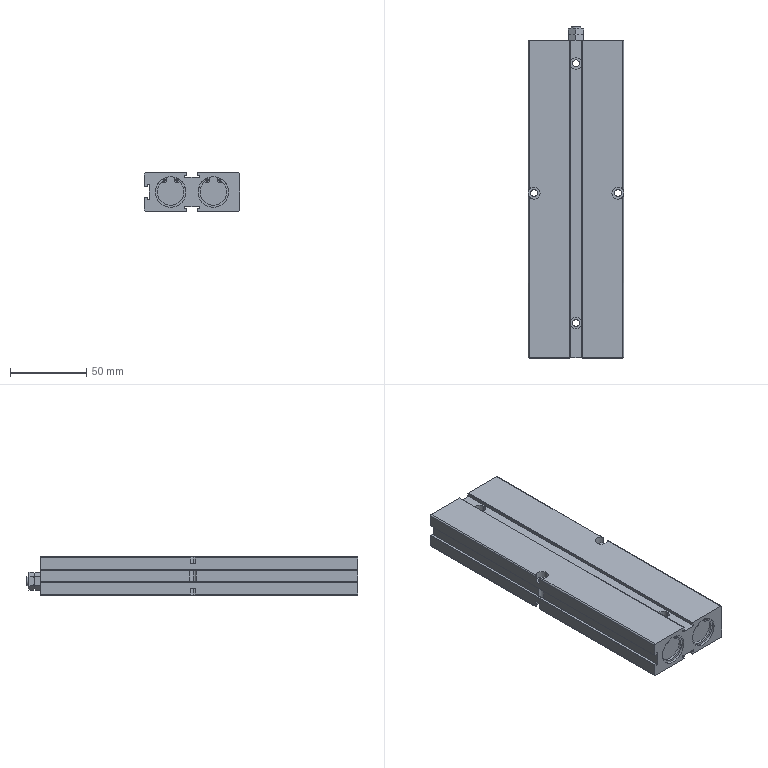Part | SolidWorks | features BaseBody 1 | 1 solid | 245 faces | box 62.3 x 217.5 x 25.2 mm | volume 196132 mm3 | cylinder 130 | plane 83 | cone 32 | commonest cylinder face diameters 0.4 x30 1.46 x16 3.5 x16 17.5 x12 20 x12 1.6 x8